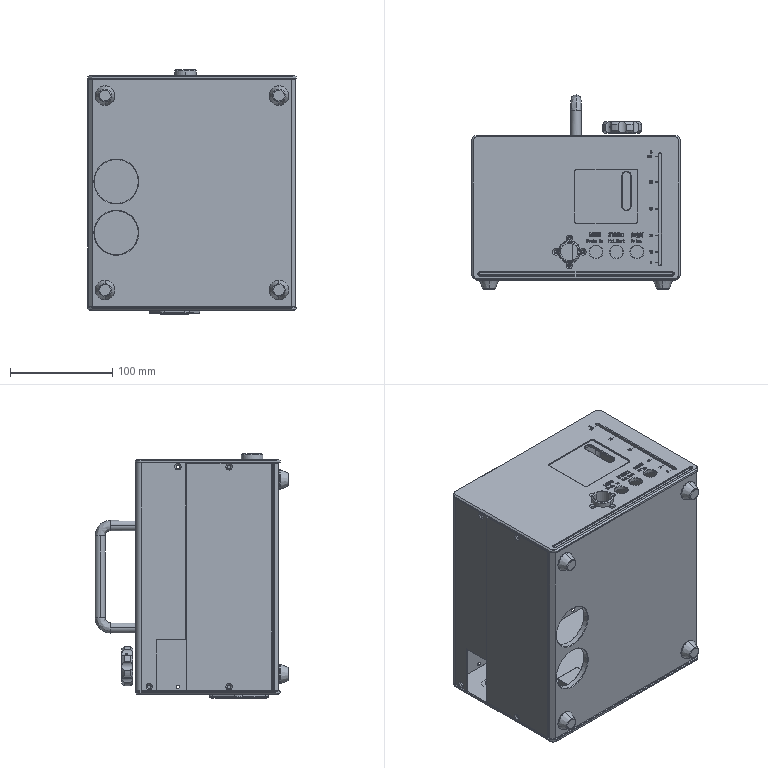Part | SolidWorks | 13 solids | 2501 faces | box 204 x 189.5 x 238.5 mm | volume 703378 mm3 | plane 1237 | spline 872 | cylinder 200 | cone 192 | commonest cylinder face diameters 3.4 x36 10 x23 0.6 x14 2.5 x14 4 x12 1 x8